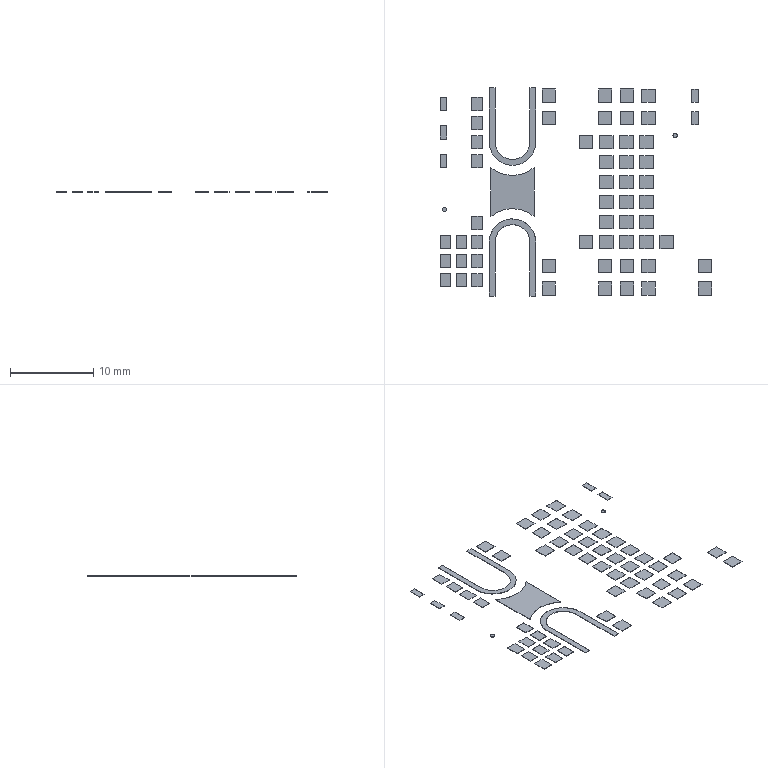Part | STEP file | 63 solids | 384 faces | box 32.638 x 25.023 x 0.05 mm | volume 9.358 mm3 | plane 372 | cylinder 12 | commonest cylinder face diameters 0.511 x4 4.201 x2 5.603 x2 4.202 x1 5.604 x1 8.033 x1